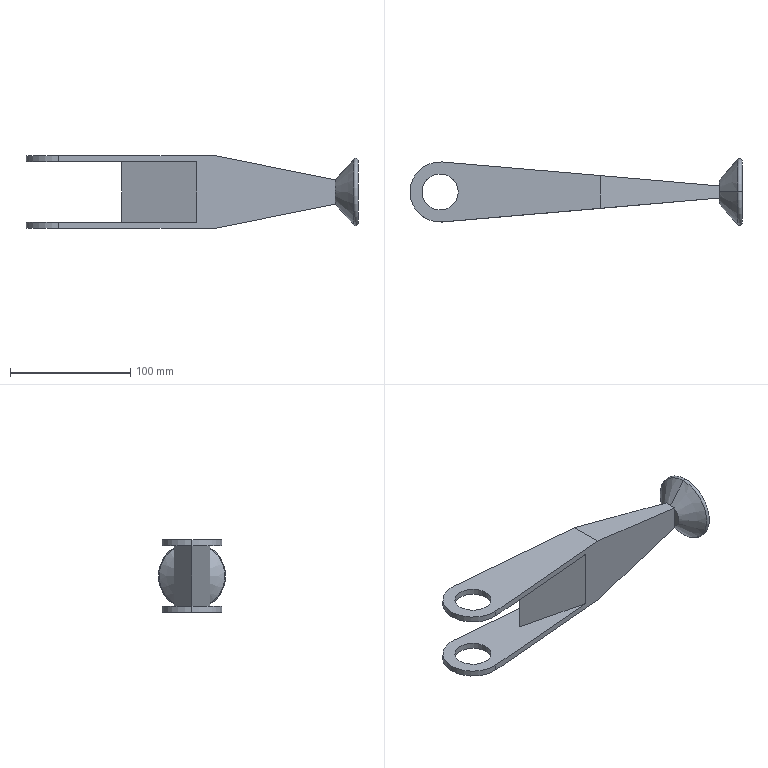Part | SolidWorks | features ICE 3, Extrusion 1, Fillet 1, Revolution 1 | 1 solid | 29 faces | box 275.852 x 55.99 x 60 mm | volume 229238 mm3 | plane 17 | cylinder 8 | torus 2 | cone 2 | commonest cylinder face diameters 30 x4 50 x4
STEP:
#1=CARTESIAN_POINT('',(247.356,0.,57.322));
#2=VERTEX_POINT('',#1);
#3=CARTESIAN_POINT('',(247.356,0.,2.678));
#4=VERTEX_POINT('',#3);
#5=CARTESIAN_POINT('',(247.356,0.,30.));
#6=DIRECTION('',(-1.,0.,0.));
#7=DIRECTION('',(0.,0.,1.));
#8=AXIS2_PLACEMENT_3D('',#5,#6,#7);
#9=CIRCLE('',#8,27.322);
#10=EDGE_CURVE('',#2,#4,#9,.T.);
#11=ORIENTED_EDGE('',*,*,#10,.F.);
#12=CARTESIAN_POINT('',(250.852,0.,55.995));
#13=VERTEX_POINT('',#12);
#14=CARTESIAN_POINT('',(248.852,0.,55.995));
#15=DIRECTION('',(0.,1.,0.));
#16=DIRECTION('',(0.,0.,1.));
#17=AXIS2_PLACEMENT_3D('',#14,#15,#16);
#18=CIRCLE('',#17,2.);
#19=EDGE_CURVE('',#2,#13,#18,.T.);
#20=ORIENTED_EDGE('',*,*,#19,.T.);
#21=CARTESIAN_POINT('',(250.852,0.,4.005));
#22=VERTEX_POINT('',#21);
#23=CARTESIAN_POINT('',(250.852,0.,30.));
#24=DIRECTION('',(1.,0.,0.));
#25=DIRECTION('',(0.,0.,-1.));
#26=AXIS2_PLACEMENT_3D('',#23,#24,#25);
#27=CIRCLE('',#26,25.995);
#28=EDGE_CURVE('',#22,#13,#27,.T.);
#29=ORIENTED_EDGE('',*,*,#28,.F.);
#30=CARTESIAN_POINT('',(248.852,0.,4.005));
#31=DIRECTION('',(0.,-1.,0.));
#32=DIRECTION('',(0.,0.,-1.));
#33=AXIS2_PLACEMENT_3D('',#30,#31,#32);
#34=CIRCLE('',#33,2.);
#35=EDGE_CURVE('',#4,#22,#34,.T.);
#36=ORIENTED_EDGE('',*,*,#35,.F.);
#37=EDGE_LOOP('',(#11,#20,#29,#36));
#38=FACE_OUTER_BOUND('',#37,.T.);
#39=CARTESIAN_POINT('',(248.852,0.,30.));
#40=DIRECTION('',(1.,0.,0.));
#41=DIRECTION('',(0.,0.,-1.));
#42=AXIS2_PLACEMENT_3D('',#39,#40,#41);
#43=TOROIDAL_SURFACE('',#42,25.995,2.);
#44=ADVANCED_FACE('',(#38),#43,.T.);
#45=CARTESIAN_POINT('',(232.,5.,38.66));
#46=VERTEX_POINT('',#45);
#47=CARTESIAN_POINT('',(232.,0.,40.));
#48=VERTEX_POINT('',#47);
#49=CARTESIAN_POINT('',(232.,0.,30.));
#50=DIRECTION('',(1.,0.,0.));
#51=DIRECTION('',(0.,0.,-1.));
#52=AXIS2_PLACEMENT_3D('',#49,#50,#51);
#53=CIRCLE('',#52,10.);
#54=EDGE_CURVE('',#46,#48,#53,.T.);
#55=ORIENTED_EDGE('',*,*,#54,.T.);
#56=CARTESIAN_POINT('',(250.852,0.,61.266));
#57=DIRECTION('',(0.6634,0.,0.7483));
#58=VECTOR('',#57,1000.);
#59=LINE('',#56,#58);
#60=EDGE_CURVE('',#48,#2,#59,.T.);
#61=ORIENTED_EDGE('',*,*,#60,.T.);
#62=ORIENTED_EDGE('',*,*,#10,.T.);
#63=CARTESIAN_POINT('',(232.,0.,20.));
#64=VERTEX_POINT('',#63);
#65=CARTESIAN_POINT('',(250.852,0.,-1.266));
#66=DIRECTION('',(0.6634,0.,-0.7483));
#67=VECTOR('',#66,1000.);
#68=LINE('',#65,#67);
#69=EDGE_CURVE('',#64,#4,#68,.T.);
#70=ORIENTED_EDGE('',*,*,#69,.F.);
#71=CARTESIAN_POINT('',(232.,5.,21.34));
#72=VERTEX_POINT('',#71);
#73=CARTESIAN_POINT('',(232.,0.,30.));
#74=DIRECTION('',(1.,0.,0.));
#75=DIRECTION('',(0.,0.,-1.));
#76=AXIS2_PLACEMENT_3D('',#73,#74,#75);
#77=CIRCLE('',#76,10.);
#78=EDGE_CURVE('',#64,#72,#77,.T.);
#79=ORIENTED_EDGE('',*,*,#78,.T.);
#80=CARTESIAN_POINT('',(232.,0.,30.));
#81=DIRECTION('',(1.,0.,0.));
#82=DIRECTION('',(0.,0.,-1.));
#83=AXIS2_PLACEMENT_3D('',#80,#81,#82);
#84=CIRCLE('',#83,10.);
#85=EDGE_CURVE('',#72,#46,#84,.T.);
#86=ORIENTED_EDGE('',*,*,#85,.T.);
#87=EDGE_LOOP('',(#55,#61,#62,#70,#79,#86));
#88=FACE_OUTER_BOUND('',#87,.T.);
#89=CARTESIAN_POINT('',(250.852,0.,30.));
#90=DIRECTION('',(1.,0.,0.));
#91=DIRECTION('',(0.,0.,-1.));
#92=AXIS2_PLACEMENT_3D('',#89,#90,#91);
#93=CONICAL_SURFACE('',#92,31.266,0.8455);
#94=ADVANCED_FACE('',(#88),#93,.T.);
#95=CARTESIAN_POINT('',(-15.,0.,60.));
#96=VERTEX_POINT('',#95);
#97=CARTESIAN_POINT('',(15.,0.,60.));
#98=VERTEX_POINT('',#97);
#99=CARTESIAN_POINT('',(0.,0.,60.));
#100=DIRECTION('',(0.,0.,1.));
#101=DIRECTION('',(1.,0.,0.));
#102=AXIS2_PLACEMENT_3D('',#99,#100,#101);
#103=CIRCLE('',#102,15.);
#104=EDGE_CURVE('',#96,#98,#103,.T.);
#105=ORIENTED_EDGE('',*,*,#104,.T.);
#106=CARTESIAN_POINT('',(15.,0.,55.));
#107=VERTEX_POINT('',#106);
#108=CARTESIAN_POINT('',(15.,0.,60.));
#109=DIRECTION('',(0.,0.,-1.));
#110=VECTOR('',#109,1000.);
#111=LINE('',#108,#110);
#112=EDGE_CURVE('',#98,#107,#111,.T.);
#113=ORIENTED_EDGE('',*,*,#112,.T.);
#114=CARTESIAN_POINT('',(-15.,0.,55.));
#115=VERTEX_POINT('',#114);
#116=CARTESIAN_POINT('',(0.,0.,55.));
#117=DIRECTION('',(0.,0.,1.));
#118=DIRECTION('',(1.,0.,0.));
#119=AXIS2_PLACEMENT_3D('',#116,#117,#118);
#120=CIRCLE('',#119,15.);
#121=EDGE_CURVE('',#115,#107,#120,.T.);
#122=ORIENTED_EDGE('',*,*,#121,.F.);
#123=CARTESIAN_POINT('',(-15.,0.,60.));
#124=DIRECTION('',(0.,0.,-1.));
#125=VECTOR('',#124,1000.);
#126=LINE('',#123,#125);
#127=EDGE_CURVE('',#96,#115,#126,.T.);
#128=ORIENTED_EDGE('',*,*,#127,.F.);
#129=EDGE_LOOP('',(#105,#113,#122,#128));
#130=FACE_OUTER_BOUND('',#129,.T.);
#131=CARTESIAN_POINT('',(0.,0.,60.));
#132=DIRECTION('',(0.,0.,-1.));
#133=DIRECTION('',(-1.,0.,0.));
#134=AXIS2_PLACEMENT_3D('',#131,#132,#133);
#135=CYLINDRICAL_SURFACE('',#134,15.);
#136=ADVANCED_FACE('',(#130),#135,.F.);
#137=CARTESIAN_POINT('',(-25.,0.,60.));
#138=VERTEX_POINT('',#137);
#139=CARTESIAN_POINT('',(2.157,-24.907,60.));
#140=VERTEX_POINT('',#139);
#141=CARTESIAN_POINT('',(0.,0.,60.));
#142=DIRECTION('',(0.,0.,1.));
#143=DIRECTION('',(1.,0.,0.));
#144=AXIS2_PLACEMENT_3D('',#141,#142,#143);
#145=CIRCLE('',#144,25.);
#146=EDGE_CURVE('',#138,#140,#145,.T.);
#147=ORIENTED_EDGE('',*,*,#146,.F.);
#148=CARTESIAN_POINT('',(-25.,0.,55.));
#149=VERTEX_POINT('',#148);
#150=CARTESIAN_POINT('',(-25.,0.,60.));
#151=DIRECTION('',(0.,0.,-1.));
#152=VECTOR('',#151,1000.);
#153=LINE('',#150,#152);
#154=EDGE_CURVE('',#138,#149,#153,.T.);
#155=ORIENTED_EDGE('',*,*,#154,.T.);
#156=CARTESIAN_POINT('',(2.157,-24.907,55.));
#157=VERTEX_POINT('',#156);
#158=CARTESIAN_POINT('',(0.,0.,55.));
#159=DIRECTION('',(0.,0.,1.));
#160=DIRECTION('',(1.,0.,0.));
#161=AXIS2_PLACEMENT_3D('',#158,#159,#160);
#162=CIRCLE('',#161,25.);
#163=EDGE_CURVE('',#149,#157,#162,.T.);
#164=ORIENTED_EDGE('',*,*,#163,.T.);
#165=CARTESIAN_POINT('',(2.157,-24.907,60.));
#166=DIRECTION('',(0.,0.,-1.));
#167=VECTOR('',#166,1000.);
#168=LINE('',#165,#167);
#169=EDGE_CURVE('',#140,#157,#168,.T.);
#170=ORIENTED_EDGE('',*,*,#169,.F.);
#171=EDGE_LOOP('',(#147,#155,#164,#170));
#172=FACE_OUTER_BOUND('',#171,.T.);
#173=CARTESIAN_POINT('',(0.,0.,60.));
#174=DIRECTION('',(0.,0.,-1.));
#175=DIRECTION('',(-1.,0.,0.));
#176=AXIS2_PLACEMENT_3D('',#173,#174,#175);
#177=CYLINDRICAL_SURFACE('',#176,25.);
#178=ADVANCED_FACE('',(#172),#177,.T.);
#179=CARTESIAN_POINT('',(-15.,0.,5.));
#180=VERTEX_POINT('',#179);
#181=CARTESIAN_POINT('',(15.,0.,5.));
#182=VERTEX_POINT('',#181);
#183=CARTESIAN_POINT('',(0.,0.,5.));
#184=DIRECTION('',(0.,0.,1.));
#185=DIRECTION('',(1.,0.,0.));
#186=AXIS2_PLACEMENT_3D('',#183,#184,#185);
#187=CIRCLE('',#186,15.);
#188=EDGE_CURVE('',#180,#182,#187,.T.);
#189=ORIENTED_EDGE('',*,*,#188,.T.);
#190=CARTESIAN_POINT('',(15.,0.,0.));
#191=VERTEX_POINT('',#190);
#192=CARTESIAN_POINT('',(15.,0.,5.));
#193=DIRECTION('',(0.,0.,-1.));
#194=VECTOR('',#193,1000.);
#195=LINE('',#192,#194);
#196=EDGE_CURVE('',#182,#191,#195,.T.);
#197=ORIENTED_EDGE('',*,*,#196,.T.);
#198=CARTESIAN_POINT('',(-15.,0.,0.));
#199=VERTEX_POINT('',#198);
#200=CARTESIAN_POINT('',(0.,0.,0.));
#201=DIRECTION('',(0.,0.,1.));
#202=DIRECTION('',(1.,0.,0.));
#203=AXIS2_PLACEMENT_3D('',#200,#201,#202);
#204=CIRCLE('',#203,15.);
#205=EDGE_CURVE('',#199,#191,#204,.T.);
#206=ORIENTED_EDGE('',*,*,#205,.F.);
#207=CARTESIAN_POINT('',(-15.,0.,5.));
#208=DIRECTION('',(0.,0.,-1.));
#209=VECTOR('',#208,1000.);
#210=LINE('',#207,#209);
#211=EDGE_CURVE('',#180,#199,#210,.T.);
#212=ORIENTED_EDGE('',*,*,#211,.F.);
#213=EDGE_LOOP('',(#189,#197,#206,#212));
#214=FACE_OUTER_BOUND('',#213,.T.);
#215=CARTESIAN_POINT('',(0.,0.,5.));
#216=DIRECTION('',(0.,0.,-1.));
#217=DIRECTION('',(-1.,0.,0.));
#218=AXIS2_PLACEMENT_3D('',#215,#216,#217);
#219=CYLINDRICAL_SURFACE('',#218,15.);
#220=ADVANCED_FACE('',(#214),#219,.F.);
#221=CARTESIAN_POINT('',(-25.,0.,5.));
#222=VERTEX_POINT('',#221);
#223=CARTESIAN_POINT('',(2.157,-24.907,5.));
#224=VERTEX_POINT('',#223);
#225=CARTESIAN_POINT('',(0.,0.,5.));
#226=DIRECTION('',(0.,0.,1.));
#227=DIRECTION('',(1.,0.,0.));
#228=AXIS2_PLACEMENT_3D('',#225,#226,#227);
#229=CIRCLE('',#228,25.);
#230=EDGE_CURVE('',#222,#224,#229,.T.);
#231=ORIENTED_EDGE('',*,*,#230,.F.);
#232=CARTESIAN_POINT('',(-25.,0.,0.));
#233=VERTEX_POINT('',#232);
#234=CARTESIAN_POINT('',(-25.,0.,5.));
#235=DIRECTION('',(0.,0.,-1.));
#236=VECTOR('',#235,1000.);
#237=LINE('',#234,#236);
#238=EDGE_CURVE('',#222,#233,#237,.T.);
#239=ORIENTED_EDGE('',*,*,#238,.T.);
#240=CARTESIAN_POINT('',(2.157,-24.907,0.));
#241=VERTEX_POINT('',#240);
#242=CARTESIAN_POINT('',(0.,0.,0.));
#243=DIRECTION('',(0.,0.,1.));
#244=DIRECTION('',(1.,0.,0.));
#245=AXIS2_PLACEMENT_3D('',#242,#243,#244);
#246=CIRCLE('',#245,25.);
#247=EDGE_CURVE('',#233,#241,#246,.T.);
#248=ORIENTED_EDGE('',*,*,#247,.T.);
#249=CARTESIAN_POINT('',(2.157,-24.907,5.));
#250=DIRECTION('',(0.,0.,-1.));
#251=VECTOR('',#250,1000.);
#252=LINE('',#249,#251);
#253=EDGE_CURVE('',#224,#241,#252,.T.);
#254=ORIENTED_EDGE('',*,*,#253,.F.);
#255=EDGE_LOOP('',(#231,#239,#248,#254));
#256=FACE_OUTER_BOUND('',#255,.T.);
#257=CARTESIAN_POINT('',(0.,0.,5.));
#258=DIRECTION('',(0.,0.,-1.));
#259=DIRECTION('',(-1.,0.,0.));
#260=AXIS2_PLACEMENT_3D('',#257,#258,#259);
#261=CYLINDRICAL_SURFACE('',#260,25.);
#262=ADVANCED_FACE('',(#256),#261,.T.);
#263=ORIENTED_EDGE('',*,*,#54,.F.);
#264=CARTESIAN_POINT('',(232.,5.,40.));
#265=VERTEX_POINT('',#264);
#266=CARTESIAN_POINT('',(232.,5.,5.));
#267=DIRECTION('',(0.,0.,-1.));
#268=VECTOR('',#267,1000.);
#269=LINE('',#266,#268);
#270=EDGE_CURVE('',#265,#46,#269,.T.);
#271=ORIENTED_EDGE('',*,*,#270,.F.);
#272=CARTESIAN_POINT('',(232.,-41.5,40.));
#273=DIRECTION('',(0.,1.,0.));
#274=VECTOR('',#273,1000.);
#275=LINE('',#272,#274);
#276=EDGE_CURVE('',#48,#265,#275,.T.);
#277=ORIENTED_EDGE('',*,*,#276,.F.);
#278=EDGE_LOOP('',(#263,#271,#277));
#279=FACE_OUTER_BOUND('',#278,.T.);
#280=CARTESIAN_POINT('',(232.,5.,5.));
#281=DIRECTION('',(-1.,0.,0.));
#282=DIRECTION('',(0.,0.,1.));
#283=AXIS2_PLACEMENT_3D('',#280,#281,#282);
#284=PLANE('',#283);
#285=ADVANCED_FACE('',(#279),#284,.F.);
#286=CARTESIAN_POINT('',(232.,-5.,38.66));
#287=VERTEX_POINT('',#286);
#288=CARTESIAN_POINT('',(232.,0.,30.));
#289=DIRECTION('',(1.,0.,0.));
#290=DIRECTION('',(0.,0.,-1.));
#291=AXIS2_PLACEMENT_3D('',#288,#289,#290);
#292=CIRCLE('',#291,10.);
#293=EDGE_CURVE('',#48,#287,#292,.T.);
#294=ORIENTED_EDGE('',*,*,#293,.F.);
#295=CARTESIAN_POINT('',(232.,-5.,40.));
#296=VERTEX_POINT('',#295);
#297=CARTESIAN_POINT('',(232.,-41.5,40.));
#298=DIRECTION('',(0.,1.,0.));
#299=VECTOR('',#298,1000.);
#300=LINE('',#297,#299);
#301=EDGE_CURVE('',#296,#48,#300,.T.);
#302=ORIENTED_EDGE('',*,*,#301,.F.);
#303=CARTESIAN_POINT('',(232.,-5.,5.));
#304=DIRECTION('',(0.,0.,-1.));
#305=VECTOR('',#304,1000.);
#306=LINE('',#303,#305);
#307=EDGE_CURVE('',#296,#287,#306,.T.);
#308=ORIENTED_EDGE('',*,*,#307,.T.);
#309=EDGE_LOOP('',(#294,#302,#308));
#310=FACE_OUTER_BOUND('',#309,.T.);
#311=CARTESIAN_POINT('',(232.,5.,5.));
#312=DIRECTION('',(-1.,0.,0.));
#313=DIRECTION('',(0.,0.,1.));
#314=AXIS2_PLACEMENT_3D('',#311,#312,#313);
#315=PLANE('',#314);
#316=ADVANCED_FACE('',(#310),#315,.F.);
#317=ORIENTED_EDGE('',*,*,#78,.F.);
#318=CARTESIAN_POINT('',(232.,5.,20.));
#319=VERTEX_POINT('',#318);
#320=CARTESIAN_POINT('',(232.,-41.5,20.));
#321=DIRECTION('',(0.,1.,0.));
#322=VECTOR('',#321,1000.);
#323=LINE('',#320,#322);
#324=EDGE_CURVE('',#64,#319,#323,.T.);
#325=ORIENTED_EDGE('',*,*,#324,.T.);
#326=CARTESIAN_POINT('',(232.,5.,5.));
#327=DIRECTION('',(0.,0.,-1.));
#328=VECTOR('',#327,1000.);
#329=LINE('',#326,#328);
#330=EDGE_CURVE('',#72,#319,#329,.T.);
#331=ORIENTED_EDGE('',*,*,#330,.F.);
#332=EDGE_LOOP('',(#317,#325,#331));
#333=FACE_OUTER_BOUND('',#332,.T.);
#334=CARTESIAN_POINT('',(232.,5.,5.));
#335=DIRECTION('',(-1.,0.,0.));
#336=DIRECTION('',(0.,0.,1.));
#337=AXIS2_PLACEMENT_3D('',#334,#335,#336);
#338=PLANE('',#337);
#339=ADVANCED_FACE('',(#333),#338,.F.);
#340=CARTESIAN_POINT('',(54.589,0.,5.));
#341=VERTEX_POINT('',#340);
#342=CARTESIAN_POINT('',(117.079,-14.953,5.));
#343=VERTEX_POINT('',#342);
#344=CARTESIAN_POINT('',(54.589,0.,5.));
#345=DIRECTION('',(0.9725,-0.2327,0.));
#346=VECTOR('',#345,1000.);
#347=LINE('',#344,#346);
#348=EDGE_CURVE('',#341,#343,#347,.T.);
#349=ORIENTED_EDGE('',*,*,#348,.F.);
#350=CARTESIAN_POINT('',(117.079,14.953,5.));
#351=VERTEX_POINT('',#350);
#352=CARTESIAN_POINT('',(117.079,14.953,5.));
#353=DIRECTION('',(-0.9725,-0.2327,0.));
#354=VECTOR('',#353,1000.);
#355=LINE('',#352,#354);
#356=EDGE_CURVE('',#351,#341,#355,.T.);
#357=ORIENTED_EDGE('',*,*,#356,.F.);
#358=CARTESIAN_POINT('',(2.157,24.907,5.));
#359=VERTEX_POINT('',#358);
#360=CARTESIAN_POINT('',(2.157,24.907,5.));
#361=DIRECTION('',(-0.9963,0.08629,0.));
#362=VECTOR('',#361,1000.);
#363=LINE('',#360,#362);
#364=EDGE_CURVE('',#351,#359,#363,.T.);
#365=ORIENTED_EDGE('',*,*,#364,.T.);
#366=CARTESIAN_POINT('',(0.,0.,5.));
#367=DIRECTION('',(0.,0.,1.));
#368=DIRECTION('',(1.,0.,0.));
#369=AXIS2_PLACEMENT_3D('',#366,#367,#368);
#370=CIRCLE('',#369,25.);
#371=EDGE_CURVE('',#359,#222,#370,.T.);
#372=ORIENTED_EDGE('',*,*,#371,.T.);
#373=ORIENTED_EDGE('',*,*,#230,.T.);
#374=CARTESIAN_POINT('',(2.157,-24.907,5.));
#375=DIRECTION('',(0.9963,0.08629,0.));
#376=VECTOR('',#375,1000.);
#377=LINE('',#374,#376);
#378=EDGE_CURVE('',#224,#343,#377,.T.);
#379=ORIENTED_EDGE('',*,*,#378,.T.);
#380=EDGE_LOOP('',(#349,#357,#365,#372,#373,#379));
#381=FACE_OUTER_BOUND('',#380,.T.);
#382=ORIENTED_EDGE('',*,*,#188,.F.);
#383=CARTESIAN_POINT('',(0.,0.,5.));
#384=DIRECTION('',(0.,0.,1.));
#385=DIRECTION('',(1.,0.,0.));
#386=AXIS2_PLACEMENT_3D('',#383,#384,#385);
#387=CIRCLE('',#386,15.);
#388=EDGE_CURVE('',#182,#180,#387,.T.);
#389=ORIENTED_EDGE('',*,*,#388,.F.);
#390=EDGE_LOOP('',(#382,#389));
#391=FACE_BOUND('',#390,.T.);
#392=CARTESIAN_POINT('',(0.,0.,5.));
#393=DIRECTION('',(0.,0.,1.));
#394=DIRECTION('',(1.,0.,0.));
#395=AXIS2_PLACEMENT_3D('',#392,#393,#394);
#396=PLANE('',#395);
#397=ADVANCED_FACE('',(#381,#391),#396,.T.);
#398=CARTESIAN_POINT('',(133.012,13.573,0.));
#399=VERTEX_POINT('',#398);
#400=CARTESIAN_POINT('',(2.157,24.907,0.));
#401=VERTEX_POINT('',#400);
#402=CARTESIAN_POINT('',(2.157,24.907,0.));
#403=DIRECTION('',(-0.9963,0.08629,0.));
#404=VECTOR('',#403,1000.);
#405=LINE('',#402,#404);
#406=EDGE_CURVE('',#399,#401,#405,.T.);
#407=ORIENTED_EDGE('',*,*,#406,.F.);
#408=CARTESIAN_POINT('',(133.012,-13.573,0.));
#409=VERTEX_POINT('',#408);
#410=CARTESIAN_POINT('',(133.012,-41.5,0.));
#411=DIRECTION('',(0.,1.,0.));
#412=VECTOR('',#411,1000.);
#413=LINE('',#410,#412);
#414=EDGE_CURVE('',#409,#399,#413,.T.);
#415=ORIENTED_EDGE('',*,*,#414,.F.);
#416=CARTESIAN_POINT('',(2.157,-24.907,0.));
#417=DIRECTION('',(0.9963,0.08629,0.));
#418=VECTOR('',#417,1000.);
#419=LINE('',#416,#418);
#420=EDGE_CURVE('',#241,#409,#419,.T.);
#421=ORIENTED_EDGE('',*,*,#420,.F.);
#422=ORIENTED_EDGE('',*,*,#247,.F.);
#423=CARTESIAN_POINT('',(0.,0.,0.));
#424=DIRECTION('',(0.,0.,1.));
#425=DIRECTION('',(1.,0.,0.));
#426=AXIS2_PLACEMENT_3D('',#423,#424,#425);
#427=CIRCLE('',#426,25.);
#428=EDGE_CURVE('',#401,#233,#427,.T.);
#429=ORIENTED_EDGE('',*,*,#428,.F.);
#430=EDGE_LOOP('',(#407,#415,#421,#422,#429));
#431=FACE_OUTER_BOUND('',#430,.T.);
#432=ORIENTED_EDGE('',*,*,#205,.T.);
#433=CARTESIAN_POINT('',(0.,0.,0.));
#434=DIRECTION('',(0.,0.,1.));
#435=DIRECTION('',(1.,0.,0.));
#436=AXIS2_PLACEMENT_3D('',#433,#434,#435);
#437=CIRCLE('',#436,15.);
#438=EDGE_CURVE('',#191,#199,#437,.T.);
#439=ORIENTED_EDGE('',*,*,#438,.T.);
#440=EDGE_LOOP('',(#432,#439));
#441=FACE_BOUND('',#440,.T.);
#442=CARTESIAN_POINT('',(0.,0.,0.));
#443=DIRECTION('',(0.,0.,1.));
#444=DIRECTION('',(1.,0.,0.));
#445=AXIS2_PLACEMENT_3D('',#442,#443,#444);
#446=PLANE('',#445);
#447=ADVANCED_FACE('',(#431,#441),#446,.F.);
#448=ORIENTED_EDGE('',*,*,#238,.F.);
#449=ORIENTED_EDGE('',*,*,#371,.F.);
#450=CARTESIAN_POINT('',(2.157,24.907,5.));
#451=DIRECTION('',(0.,0.,-1.));
#452=VECTOR('',#451,1000.);
#453=LINE('',#450,#452);
#454=EDGE_CURVE('',#359,#401,#453,.T.);
#455=ORIENTED_EDGE('',*,*,#454,.T.);
#456=ORIENTED_EDGE('',*,*,#428,.T.);
#457=EDGE_LOOP('',(#448,#449,#455,#456));
#458=FACE_OUTER_BOUND('',#457,.T.);
#459=CARTESIAN_POINT('',(0.,0.,5.));
#460=DIRECTION('',(0.,0.,-1.));
#461=DIRECTION('',(-1.,0.,0.));
#462=AXIS2_PLACEMENT_3D('',#459,#460,#461);
#463=CYLINDRICAL_SURFACE('',#462,25.);
#464=ADVANCED_FACE('',(#458),#463,.T.);
#465=ORIENTED_EDGE('',*,*,#420,.T.);
#466=CARTESIAN_POINT('',(232.,-5.,20.));
#467=VERTEX_POINT('',#466);
#468=CARTESIAN_POINT('',(8.216,-24.382,-25.214));
#469=DIRECTION('',(0.9767,0.08459,0.1973));
#470=VECTOR('',#469,1000.);
#471=LINE('',#468,#470);
#472=EDGE_CURVE('',#409,#467,#471,.T.);
#473=ORIENTED_EDGE('',*,*,#472,.T.);
#474=CARTESIAN_POINT('',(232.,-5.,21.34));
#475=VERTEX_POINT('',#474);
#476=CARTESIAN_POINT('',(232.,-5.,5.));
#477=DIRECTION('',(0.,0.,-1.));
#478=VECTOR('',#477,1000.);
#479=LINE('',#476,#478);
#480=EDGE_CURVE('',#475,#467,#479,.T.);
#481=ORIENTED_EDGE('',*,*,#480,.F.);
#482=CARTESIAN_POINT('',(232.,-5.,5.));
#483=DIRECTION('',(0.,0.,-1.));
#484=VECTOR('',#483,1000.);
#485=LINE('',#482,#484);
#486=EDGE_CURVE('',#287,#475,#485,.T.);
#487=ORIENTED_EDGE('',*,*,#486,.F.);
#488=ORIENTED_EDGE('',*,*,#307,.F.);
#489=CARTESIAN_POINT('',(133.012,-13.573,60.));
#490=VERTEX_POINT('',#489);
#491=CARTESIAN_POINT('',(17.853,-23.547,83.267));
#492=DIRECTION('',(-0.9767,-0.08459,0.1973));
#493=VECTOR('',#492,1000.);
#494=LINE('',#491,#493);
#495=EDGE_CURVE('',#296,#490,#494,.T.);
#496=ORIENTED_EDGE('',*,*,#495,.T.);
#497=CARTESIAN_POINT('',(117.079,-14.953,60.));
#498=DIRECTION('',(0.9963,0.08629,0.));
#499=VECTOR('',#498,1000.);
#500=LINE('',#497,#499);
#501=EDGE_CURVE('',#140,#490,#500,.T.);
#502=ORIENTED_EDGE('',*,*,#501,.F.);
#503=ORIENTED_EDGE('',*,*,#169,.T.);
#504=CARTESIAN_POINT('',(117.079,-14.953,55.));
#505=VERTEX_POINT('',#504);
#506=CARTESIAN_POINT('',(2.157,-24.907,55.));
#507=DIRECTION('',(0.9963,0.08629,0.));
#508=VECTOR('',#507,1000.);
#509=LINE('',#506,#508);
#510=EDGE_CURVE('',#157,#505,#509,.T.);
#511=ORIENTED_EDGE('',*,*,#510,.T.);
#512=CARTESIAN_POINT('',(117.079,-14.953,55.));
#513=DIRECTION('',(0.,0.,-1.));
#514=VECTOR('',#513,1000.);
#515=LINE('',#512,#514);
#516=EDGE_CURVE('',#505,#343,#515,.T.);
#517=ORIENTED_EDGE('',*,*,#516,.T.);
#518=ORIENTED_EDGE('',*,*,#378,.F.);
#519=ORIENTED_EDGE('',*,*,#253,.T.);
#520=EDGE_LOOP('',(#465,#473,#481,#487,#488,#496,#502,#503,#511,#517,#518,#519));
#521=FACE_OUTER_BOUND('',#520,.T.);
#522=CARTESIAN_POINT('',(2.157,-24.907,5.));
#523=DIRECTION('',(-0.08629,0.9963,0.));
#524=DIRECTION('',(-0.9963,-0.08629,0.));
#525=AXIS2_PLACEMENT_3D('',#522,#523,#524);
#526=PLANE('',#525);
#527=ADVANCED_FACE('',(#521),#526,.F.);
#528=CARTESIAN_POINT('',(232.,0.,30.));
#529=DIRECTION('',(1.,0.,0.));
#530=DIRECTION('',(0.,0.,-1.));
#531=AXIS2_PLACEMENT_3D('',#528,#529,#530);
#532=CIRCLE('',#531,10.);
#533=EDGE_CURVE('',#475,#64,#532,.T.);
#534=ORIENTED_EDGE('',*,*,#533,.F.);
#535=ORIENTED_EDGE('',*,*,#480,.T.);
#536=CARTESIAN_POINT('',(232.,-41.5,20.));
#537=DIRECTION('',(0.,1.,0.));
#538=VECTOR('',#537,1000.);
#539=LINE('',#536,#538);
#540=EDGE_CURVE('',#467,#64,#539,.T.);
#541=ORIENTED_EDGE('',*,*,#540,.T.);
#542=EDGE_LOOP('',(#534,#535,#541));
#543=FACE_OUTER_BOUND('',#542,.T.);
#544=CARTESIAN_POINT('',(232.,5.,5.));
#545=DIRECTION('',(-1.,0.,0.));
#546=DIRECTION('',(0.,0.,1.));
#547=AXIS2_PLACEMENT_3D('',#544,#545,#546);
#548=PLANE('',#547);
#549=ADVANCED_FACE('',(#543),#548,.F.);
#550=ORIENTED_EDGE('',*,*,#270,.T.);
#551=CARTESIAN_POINT('',(232.,5.,5.));
#552=DIRECTION('',(0.,0.,-1.));
#553=VECTOR('',#552,1000.);
#554=LINE('',#551,#553);
#555=EDGE_CURVE('',#46,#72,#554,.T.);
#556=ORIENTED_EDGE('',*,*,#555,.T.);
#557=ORIENTED_EDGE('',*,*,#330,.T.);
#558=CARTESIAN_POINT('',(8.216,24.382,-25.214));
#559=DIRECTION('',(-0.9767,0.08459,-0.1973));
#560=VECTOR('',#559,1000.);
#561=LINE('',#558,#560);
#562=EDGE_CURVE('',#319,#399,#561,.T.);
#563=ORIENTED_EDGE('',*,*,#562,.T.);
#564=ORIENTED_EDGE('',*,*,#406,.T.);
#565=ORIENTED_EDGE('',*,*,#454,.F.);
#566=ORIENTED_EDGE('',*,*,#364,.F.);
#567=CARTESIAN_POINT('',(117.079,14.953,55.));
#568=VERTEX_POINT('',#567);
#569=CARTESIAN_POINT('',(117.079,14.953,55.));
#570=DIRECTION('',(0.,0.,-1.));
#571=VECTOR('',#570,1000.);
#572=LINE('',#569,#571);
#573=EDGE_CURVE('',#568,#351,#572,.T.);
#574=ORIENTED_EDGE('',*,*,#573,.F.);
#575=CARTESIAN_POINT('',(2.157,24.907,55.));
#576=VERTEX_POINT('',#575);
#577=CARTESIAN_POINT('',(117.079,14.953,55.));
#578=DIRECTION('',(-0.9963,0.08629,0.));
#579=VECTOR('',#578,1000.);
#580=LINE('',#577,#579);
#581=EDGE_CURVE('',#568,#576,#580,.T.);
#582=ORIENTED_EDGE('',*,*,#581,.T.);
#583=CARTESIAN_POINT('',(2.157,24.907,60.));
#584=VERTEX_POINT('',#583);
#585=CARTESIAN_POINT('',(2.157,24.907,60.));
#586=DIRECTION('',(0.,0.,-1.));
#587=VECTOR('',#586,1000.);
#588=LINE('',#585,#587);
#589=EDGE_CURVE('',#584,#576,#588,.T.);
#590=ORIENTED_EDGE('',*,*,#589,.F.);
#591=CARTESIAN_POINT('',(133.012,13.573,60.));
#592=VERTEX_POINT('',#591);
#593=CARTESIAN_POINT('',(232.,5.,60.));
#594=DIRECTION('',(-0.9963,0.08629,0.));
#595=VECTOR('',#594,1000.);
#596=LINE('',#593,#595);
#597=EDGE_CURVE('',#592,#584,#596,.T.);
#598=ORIENTED_EDGE('',*,*,#597,.F.);
#599=CARTESIAN_POINT('',(17.853,23.547,83.267));
#600=DIRECTION('',(0.9767,-0.08459,-0.1973));
#601=VECTOR('',#600,1000.);
#602=LINE('',#599,#601);
#603=EDGE_CURVE('',#592,#265,#602,.T.);
#604=ORIENTED_EDGE('',*,*,#603,.T.);
#605=EDGE_LOOP('',(#550,#556,#557,#563,#564,#565,#566,#574,#582,#590,#598,#604));
#606=FACE_OUTER_BOUND('',#605,.T.);
#607=CARTESIAN_POINT('',(2.157,24.907,5.));
#608=DIRECTION('',(-0.08629,-0.9963,0.));
#609=DIRECTION('',(0.9963,-0.08629,0.));
#610=AXIS2_PLACEMENT_3D('',#607,#608,#609);
#611=PLANE('',#610);
#612=ADVANCED_FACE('',(#606),#611,.F.);
#613=ORIENTED_EDGE('',*,*,#196,.F.);
#614=ORIENTED_EDGE('',*,*,#388,.T.);
#615=ORIENTED_EDGE('',*,*,#211,.T.);
#616=ORIENTED_EDGE('',*,*,#438,.F.);
#617=EDGE_LOOP('',(#613,#614,#615,#616));
#618=FACE_OUTER_BOUND('',#617,.T.);
#619=CARTESIAN_POINT('',(0.,0.,5.));
#620=DIRECTION('',(0.,0.,-1.));
#621=DIRECTION('',(-1.,0.,0.));
#622=AXIS2_PLACEMENT_3D('',#619,#620,#621);
#623=CYLINDRICAL_SURFACE('',#622,15.);
#624=ADVANCED_FACE('',(#618),#623,.F.);
#625=ORIENTED_EDGE('',*,*,#356,.T.);
#626=CARTESIAN_POINT('',(54.589,0.,55.));
#627=VERTEX_POINT('',#626);
#628=CARTESIAN_POINT('',(54.589,0.,55.));
#629=DIRECTION('',(0.,0.,-1.));
#630=VECTOR('',#629,1000.);
#631=LINE('',#628,#630);
#632=EDGE_CURVE('',#627,#341,#631,.T.);
#633=ORIENTED_EDGE('',*,*,#632,.F.);
#634=CARTESIAN_POINT('',(117.079,14.953,55.));
#635=DIRECTION('',(-0.9725,-0.2327,0.));
#636=VECTOR('',#635,1000.);
#637=LINE('',#634,#636);
#638=EDGE_CURVE('',#568,#627,#637,.T.);
#639=ORIENTED_EDGE('',*,*,#638,.F.);
#640=ORIENTED_EDGE('',*,*,#573,.T.);
#641=EDGE_LOOP('',(#625,#633,#639,#640));
#642=FACE_OUTER_BOUND('',#641,.T.);
#643=CARTESIAN_POINT('',(117.079,14.953,55.));
#644=DIRECTION('',(0.2327,-0.9725,0.));
#645=DIRECTION('',(0.9725,0.2327,0.));
#646=AXIS2_PLACEMENT_3D('',#643,#644,#645);
#647=PLANE('',#646);
#648=ADVANCED_FACE('',(#642),#647,.F.);
#649=ORIENTED_EDGE('',*,*,#348,.T.);
#650=ORIENTED_EDGE('',*,*,#516,.F.);
#651=CARTESIAN_POINT('',(54.589,0.,55.));
#652=DIRECTION('',(0.9725,-0.2327,0.));
#653=VECTOR('',#652,1000.);
#654=LINE('',#651,#653);
#655=EDGE_CURVE('',#627,#505,#654,.T.);
#656=ORIENTED_EDGE('',*,*,#655,.F.);
#657=ORIENTED_EDGE('',*,*,#632,.T.);
#658=EDGE_LOOP('',(#649,#650,#656,#657));
#659=FACE_OUTER_BOUND('',#658,.T.);
#660=CARTESIAN_POINT('',(54.589,0.,55.));
#661=DIRECTION('',(0.2327,0.9725,0.));
#662=DIRECTION('',(-0.9725,0.2327,0.));
#663=AXIS2_PLACEMENT_3D('',#660,#661,#662);
#664=PLANE('',#663);
#665=ADVANCED_FACE('',(#659),#664,.F.);
#666=ORIENTED_EDGE('',*,*,#121,.T.);
#667=CARTESIAN_POINT('',(0.,0.,55.));
#668=DIRECTION('',(0.,0.,1.));
#669=DIRECTION('',(1.,0.,0.));
#670=AXIS2_PLACEMENT_3D('',#667,#668,#669);
#671=CIRCLE('',#670,15.);
#672=EDGE_CURVE('',#107,#115,#671,.T.);
#673=ORIENTED_EDGE('',*,*,#672,.T.);
#674=EDGE_LOOP('',(#666,#673));
#675=FACE_BOUND('',#674,.T.);
#676=ORIENTED_EDGE('',*,*,#581,.F.);
#677=ORIENTED_EDGE('',*,*,#638,.T.);
#678=ORIENTED_EDGE('',*,*,#655,.T.);
#679=ORIENTED_EDGE('',*,*,#510,.F.);
#680=ORIENTED_EDGE('',*,*,#163,.F.);
#681=CARTESIAN_POINT('',(0.,0.,55.));
#682=DIRECTION('',(0.,0.,1.));
#683=DIRECTION('',(1.,0.,0.));
#684=AXIS2_PLACEMENT_3D('',#681,#682,#683);
#685=CIRCLE('',#684,25.);
#686=EDGE_CURVE('',#576,#149,#685,.T.);
#687=ORIENTED_EDGE('',*,*,#686,.F.);
#688=EDGE_LOOP('',(#676,#677,#678,#679,#680,#687));
#689=FACE_OUTER_BOUND('',#688,.T.);
#690=CARTESIAN_POINT('',(0.,0.,55.));
#691=DIRECTION('',(0.,0.,1.));
#692=DIRECTION('',(1.,0.,0.));
#693=AXIS2_PLACEMENT_3D('',#690,#691,#692);
#694=PLANE('',#693);
#695=ADVANCED_FACE('',(#675,#689),#694,.F.);
#696=CARTESIAN_POINT('',(133.012,0.,60.));
#697=DIRECTION('',(0.,-1.,0.));
#698=VECTOR('',#697,1000.);
#699=LINE('',#696,#698);
#700=EDGE_CURVE('',#592,#490,#699,.T.);
#701=ORIENTED_EDGE('',*,*,#700,.F.);
#702=ORIENTED_EDGE('',*,*,#597,.T.);
#703=CARTESIAN_POINT('',(0.,0.,60.));
#704=DIRECTION('',(0.,0.,1.));
#705=DIRECTION('',(1.,0.,0.));
#706=AXIS2_PLACEMENT_3D('',#703,#704,#705);
#707=CIRCLE('',#706,25.);
#708=EDGE_CURVE('',#584,#138,#707,.T.);
#709=ORIENTED_EDGE('',*,*,#708,.T.);
#710=ORIENTED_EDGE('',*,*,#146,.T.);
#711=ORIENTED_EDGE('',*,*,#501,.T.);
#712=EDGE_LOOP('',(#701,#702,#709,#710,#711));
#713=FACE_OUTER_BOUND('',#712,.T.);
#714=ORIENTED_EDGE('',*,*,#104,.F.);
#715=CARTESIAN_POINT('',(0.,0.,60.));
#716=DIRECTION('',(0.,0.,1.));
#717=DIRECTION('',(1.,0.,0.));
#718=AXIS2_PLACEMENT_3D('',#715,#716,#717);
#719=CIRCLE('',#718,15.);
#720=EDGE_CURVE('',#98,#96,#719,.T.);
#721=ORIENTED_EDGE('',*,*,#720,.F.);
#722=EDGE_LOOP('',(#714,#721));
#723=FACE_BOUND('',#722,.T.);
#724=CARTESIAN_POINT('',(0.,0.,60.));
#725=DIRECTION('',(0.,0.,1.));
#726=DIRECTION('',(1.,0.,0.));
#727=AXIS2_PLACEMENT_3D('',#724,#725,#726);
#728=PLANE('',#727);
#729=ADVANCED_FACE('',(#713,#723),#728,.T.);
#730=ORIENTED_EDGE('',*,*,#154,.F.);
#731=ORIENTED_EDGE('',*,*,#708,.F.);
#732=ORIENTED_EDGE('',*,*,#589,.T.);
#733=ORIENTED_EDGE('',*,*,#686,.T.);
#734=EDGE_LOOP('',(#730,#731,#732,#733));
#735=FACE_OUTER_BOUND('',#734,.T.);
#736=CARTESIAN_POINT('',(0.,0.,60.));
#737=DIRECTION('',(0.,0.,-1.));
#738=DIRECTION('',(-1.,0.,0.));
#739=AXIS2_PLACEMENT_3D('',#736,#737,#738);
#740=CYLINDRICAL_SURFACE('',#739,25.);
#741=ADVANCED_FACE('',(#735),#740,.T.);
#742=ORIENTED_EDGE('',*,*,#112,.F.);
#743=ORIENTED_EDGE('',*,*,#720,.T.);
#744=ORIENTED_EDGE('',*,*,#127,.T.);
#745=ORIENTED_EDGE('',*,*,#672,.F.);
#746=EDGE_LOOP('',(#742,#743,#744,#745));
#747=FACE_OUTER_BOUND('',#746,.T.);
#748=CARTESIAN_POINT('',(0.,0.,60.));
#749=DIRECTION('',(0.,0.,-1.));
#750=DIRECTION('',(-1.,0.,0.));
#751=AXIS2_PLACEMENT_3D('',#748,#749,#750);
#752=CYLINDRICAL_SURFACE('',#751,15.);
#753=ADVANCED_FACE('',(#747),#752,.F.);
#754=ORIENTED_EDGE('',*,*,#301,.T.);
#755=ORIENTED_EDGE('',*,*,#276,.T.);
#756=ORIENTED_EDGE('',*,*,#603,.F.);
#757=ORIENTED_EDGE('',*,*,#700,.T.);
#758=ORIENTED_EDGE('',*,*,#495,.F.);
#759=EDGE_LOOP('',(#754,#755,#756,#757,#758));
#760=FACE_OUTER_BOUND('',#759,.T.);
#761=CARTESIAN_POINT('',(133.012,-41.5,60.));
#762=DIRECTION('',(-0.198,0.,-0.9802));
#763=DIRECTION('',(-0.9802,0.,0.198));
#764=AXIS2_PLACEMENT_3D('',#761,#762,#763);
#765=PLANE('',#764);
#766=ADVANCED_FACE('',(#760),#765,.F.);
#767=ORIENTED_EDGE('',*,*,#414,.T.);
#768=ORIENTED_EDGE('',*,*,#562,.F.);
#769=ORIENTED_EDGE('',*,*,#324,.F.);
#770=ORIENTED_EDGE('',*,*,#540,.F.);
#771=ORIENTED_EDGE('',*,*,#472,.F.);
#772=EDGE_LOOP('',(#767,#768,#769,#770,#771));
#773=FACE_OUTER_BOUND('',#772,.T.);
#774=CARTESIAN_POINT('',(133.012,-41.5,0.));
#775=DIRECTION('',(-0.198,0.,0.9802));
#776=DIRECTION('',(0.9802,0.,0.198));
#777=AXIS2_PLACEMENT_3D('',#774,#775,#776);
#778=PLANE('',#777);
#779=ADVANCED_FACE('',(#773),#778,.F.);
#780=ORIENTED_EDGE('',*,*,#555,.F.);
#781=ORIENTED_EDGE('',*,*,#85,.F.);
#782=EDGE_LOOP('',(#780,#781));
#783=FACE_OUTER_BOUND('',#782,.T.);
#784=CARTESIAN_POINT('',(232.,0.,30.));
#785=DIRECTION('',(-1.,0.,0.));
#786=DIRECTION('',(0.,0.,1.));
#787=AXIS2_PLACEMENT_3D('',#784,#785,#786);
#788=PLANE('',#787);
#789=ADVANCED_FACE('',(#783),#788,.T.);
#790=CARTESIAN_POINT('',(232.,0.,30.));
#791=DIRECTION('',(1.,0.,0.));
#792=DIRECTION('',(0.,0.,-1.));
#793=AXIS2_PLACEMENT_3D('',#790,#791,#792);
#794=CIRCLE('',#793,10.);
#795=EDGE_CURVE('',#287,#475,#794,.T.);
#796=ORIENTED_EDGE('',*,*,#795,.F.);
#797=ORIENTED_EDGE('',*,*,#486,.T.);
#798=EDGE_LOOP('',(#796,#797));
#799=FACE_OUTER_BOUND('',#798,.T.);
#800=CARTESIAN_POINT('',(232.,0.,30.));
#801=DIRECTION('',(-1.,0.,0.));
#802=DIRECTION('',(0.,0.,1.));
#803=AXIS2_PLACEMENT_3D('',#800,#801,#802);
#804=PLANE('',#803);
#805=ADVANCED_FACE('',(#799),#804,.T.);
#806=ORIENTED_EDGE('',*,*,#60,.F.);
#807=ORIENTED_EDGE('',*,*,#293,.T.);
#808=ORIENTED_EDGE('',*,*,#795,.T.);
#809=ORIENTED_EDGE('',*,*,#533,.T.);
#810=ORIENTED_EDGE('',*,*,#69,.T.);
#811=CARTESIAN_POINT('',(247.356,0.,30.));
#812=DIRECTION('',(-1.,0.,0.));
#813=DIRECTION('',(0.,0.,1.));
#814=AXIS2_PLACEMENT_3D('',#811,#812,#813);
#815=CIRCLE('',#814,27.322);
#816=EDGE_CURVE('',#4,#2,#815,.T.);
#817=ORIENTED_EDGE('',*,*,#816,.T.);
#818=EDGE_LOOP('',(#806,#807,#808,#809,#810,#817));
#819=FACE_OUTER_BOUND('',#818,.T.);
#820=CARTESIAN_POINT('',(250.852,0.,30.));
#821=DIRECTION('',(1.,0.,0.));
#822=DIRECTION('',(0.,0.,-1.));
#823=AXIS2_PLACEMENT_3D('',#820,#821,#822);
#824=CONICAL_SURFACE('',#823,31.266,0.8455);
#825=ADVANCED_FACE('',(#819),#824,.T.);
#826=ORIENTED_EDGE('',*,*,#28,.T.);
#827=CARTESIAN_POINT('',(250.852,0.,30.));
#828=DIRECTION('',(1.,0.,0.));
#829=DIRECTION('',(0.,0.,-1.));
#830=AXIS2_PLACEMENT_3D('',#827,#828,#829);
#831=CIRCLE('',#830,25.995);
#832=EDGE_CURVE('',#13,#22,#831,.T.);
#833=ORIENTED_EDGE('',*,*,#832,.T.);
#834=EDGE_LOOP('',(#826,#833));
#835=FACE_OUTER_BOUND('',#834,.T.);
#836=CARTESIAN_POINT('',(250.852,0.,-1.266));
#837=DIRECTION('',(1.,0.,0.));
#838=DIRECTION('',(0.,0.,-1.));
#839=AXIS2_PLACEMENT_3D('',#836,#837,#838);
#840=PLANE('',#839);
#841=ADVANCED_FACE('',(#835),#840,.T.);
#842=ORIENTED_EDGE('',*,*,#19,.F.);
#843=ORIENTED_EDGE('',*,*,#816,.F.);
#844=ORIENTED_EDGE('',*,*,#35,.T.);
#845=ORIENTED_EDGE('',*,*,#832,.F.);
#846=EDGE_LOOP('',(#842,#843,#844,#845));
#847=FACE_OUTER_BOUND('',#846,.T.);
#848=CARTESIAN_POINT('',(248.852,0.,30.));
#849=DIRECTION('',(1.,0.,0.));
#850=DIRECTION('',(0.,0.,-1.));
#851=AXIS2_PLACEMENT_3D('',#848,#849,#850);
#852=TOROIDAL_SURFACE('',#851,25.995,2.);
#853=ADVANCED_FACE('',(#847),#852,.T.);
#854=CLOSED_SHELL('',(#44,#94,#136,#178,#220,#262,#285,#316,#339,#397,#447,#464,#527,#549,#612,#624,#648,#665,#695,#729,#741,#753,#766,#779,#789,#805,#825,#841,#853));
#855=MANIFOLD_SOLID_BREP('',#854);
#856=CARTESIAN_POINT('',(0.,0.,0.));
#857=DIRECTION('',(0.,0.,1.));
#858=DIRECTION('',(1.,0.,0.));
#859=AXIS2_PLACEMENT_3D('',#856,#857,#858);
#860=(LENGTH_UNIT()NAMED_UNIT(*)SI_UNIT(.MILLI.,.METRE.));
#861=UNCERTAINTY_MEASURE_WITH_UNIT(LENGTH_MEASURE(0.00001),#860,'','');
#862=(NAMED_UNIT(*)PLANE_ANGLE_UNIT()SI_UNIT($,.RADIAN.));
#863=(NAMED_UNIT(*)SI_UNIT($,.STERADIAN.)SOLID_ANGLE_UNIT());
#864=(GEOMETRIC_REPRESENTATION_CONTEXT(3)GLOBAL_UNCERTAINTY_ASSIGNED_CONTEXT((#861))GLOBAL_UNIT_ASSIGNED_CONTEXT((#860,#862,#863))REPRESENTATION_CONTEXT('',''));
#865=ADVANCED_BREP_SHAPE_REPRESENTATION('',(#855,#859),#864);